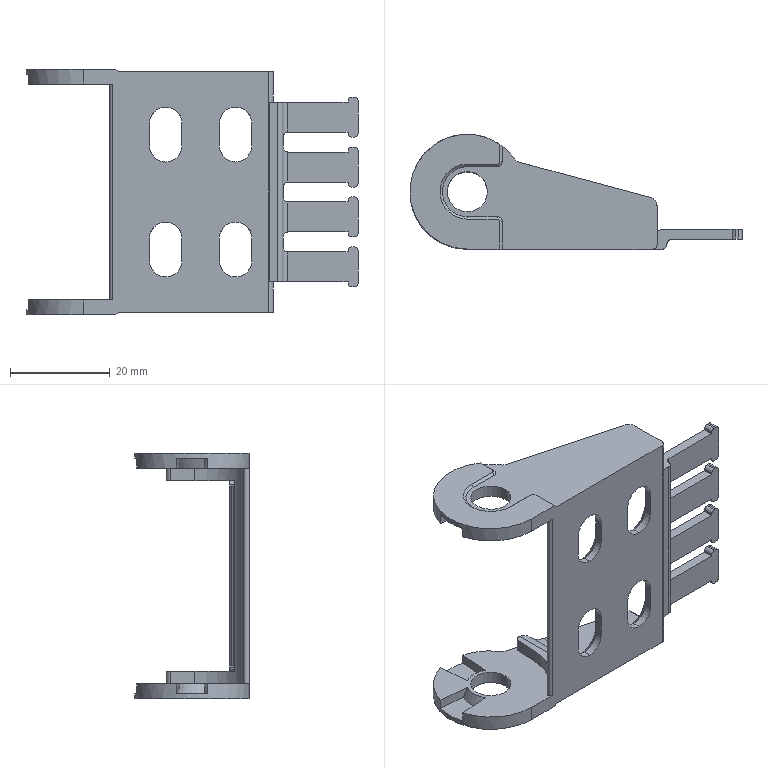Part | SolidWorks | features BaseBody 1 | 1 solid | 176 faces | box 66.5 x 23 x 49.2 mm | volume 8263 mm3 | plane 85 | cylinder 61 | cone 18 | spline 12 | commonest cylinder face diameters 1.5 x16 2 x13 6.5 x12 4 x4 8.05 x4 1.2 x3